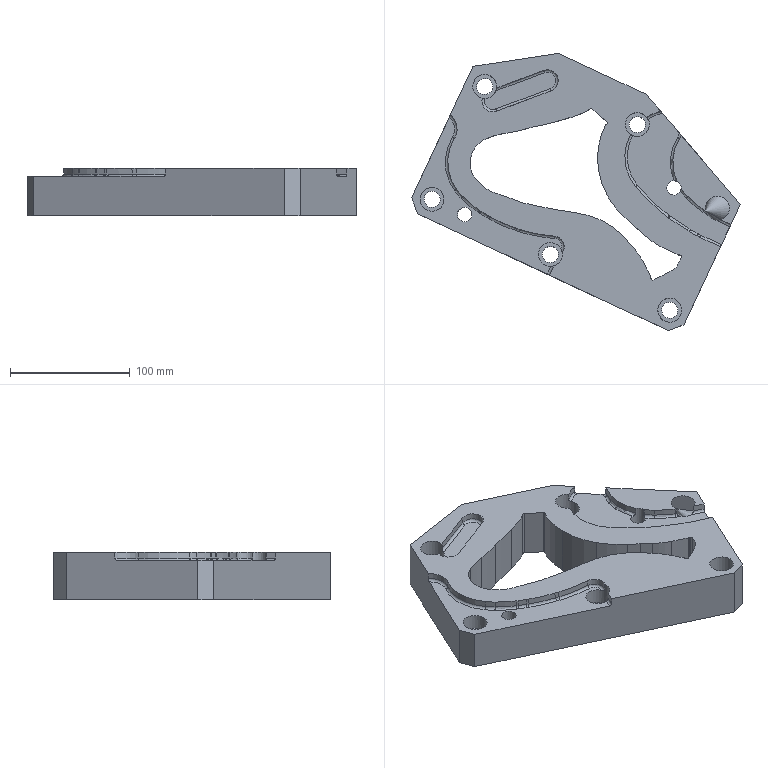Part | NX | features 23 2 | 1 solid | 152 faces | box 274.394 x 231.473 x 40 mm | volume 1101149 mm3 | cylinder 69 | spline 38 | plane 30 | torus 15 | commonest cylinder face diameters 2 x10 20 x7 13.5 x6 4 x5 30.155 x3 75.918 x3